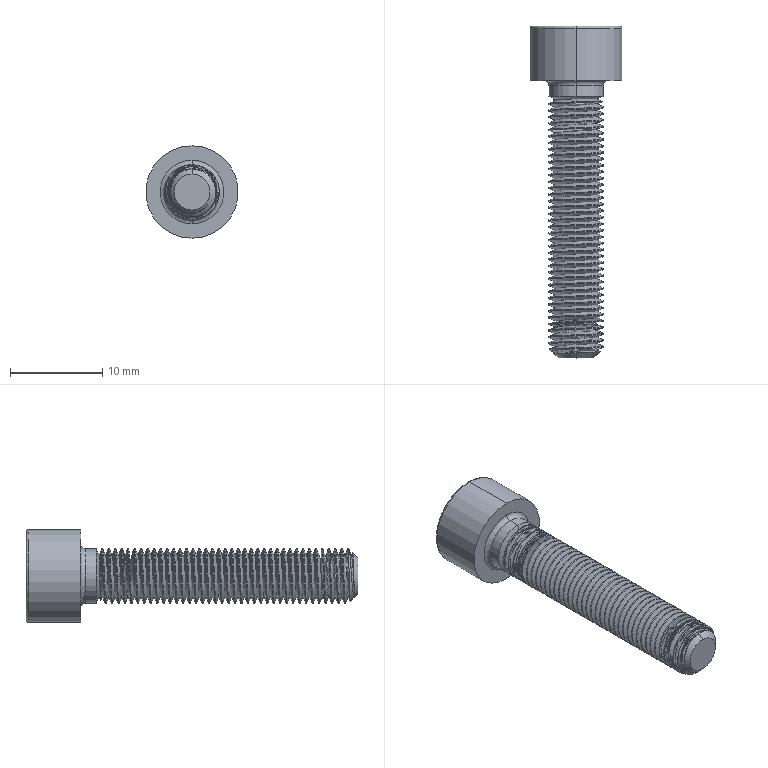Part | STEP file | Parafuso M6 - 30mm | 1 solid | 113 faces | box 10 x 35.9 x 10 mm | volume 1008 mm3 | cylinder 82 | cone 13 | plane 10 | torus 6 | spline 2 | commonest cylinder face diameters 5.9 x80 10 x2